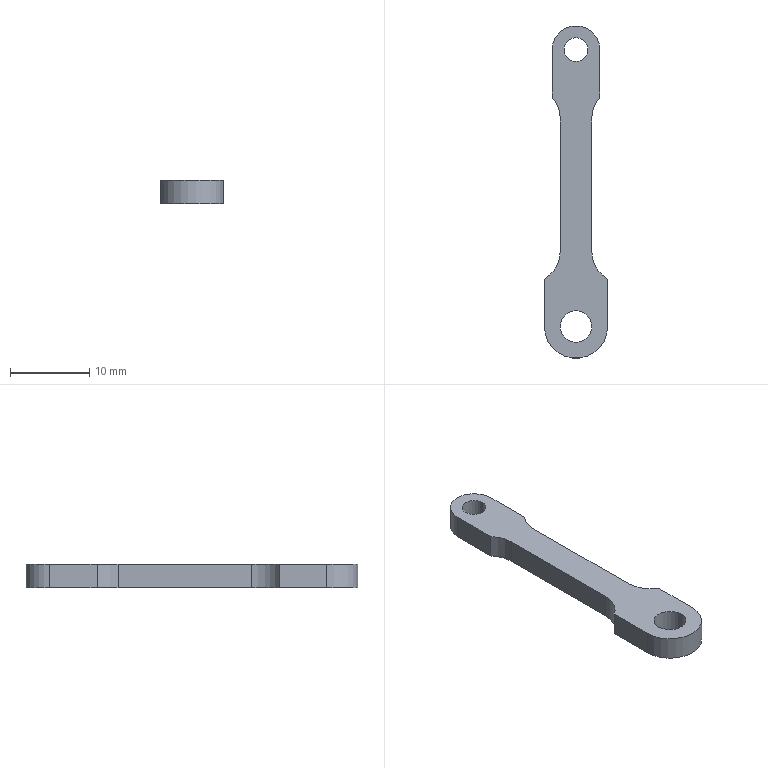Part | SolidWorks | features Extrusion 1 | 1 solid | 18 faces | box 8 x 42 x 3 mm | volume 603.988 mm3 | cylinder 10 | plane 8 | commonest cylinder face diameters 8 x5 3 x2 4 x2 6 x1
STEP:
#1=CARTESIAN_POINT('',(-2.,-35.,1.5));
#2=VERTEX_POINT('',#1);
#3=CARTESIAN_POINT('',(2.,-35.,1.5));
#4=VERTEX_POINT('',#3);
#5=CARTESIAN_POINT('',(0.,-35.,1.5));
#6=DIRECTION('',(0.,0.,1.));
#7=DIRECTION('',(1.,0.,0.));
#8=AXIS2_PLACEMENT_3D('',#5,#6,#7);
#9=CIRCLE('',#8,2.);
#10=EDGE_CURVE('',#2,#4,#9,.T.);
#11=ORIENTED_EDGE('',*,*,#10,.T.);
#12=CARTESIAN_POINT('',(2.,-35.,-1.5));
#13=VERTEX_POINT('',#12);
#14=CARTESIAN_POINT('',(2.,-35.,1.5));
#15=DIRECTION('',(0.,0.,-1.));
#16=VECTOR('',#15,1000.);
#17=LINE('',#14,#16);
#18=EDGE_CURVE('',#4,#13,#17,.T.);
#19=ORIENTED_EDGE('',*,*,#18,.T.);
#20=CARTESIAN_POINT('',(-2.,-35.,-1.5));
#21=VERTEX_POINT('',#20);
#22=CARTESIAN_POINT('',(0.,-35.,-1.5));
#23=DIRECTION('',(0.,0.,1.));
#24=DIRECTION('',(1.,0.,0.));
#25=AXIS2_PLACEMENT_3D('',#22,#23,#24);
#26=CIRCLE('',#25,2.);
#27=EDGE_CURVE('',#21,#13,#26,.T.);
#28=ORIENTED_EDGE('',*,*,#27,.F.);
#29=CARTESIAN_POINT('',(-2.,-35.,1.5));
#30=DIRECTION('',(0.,0.,-1.));
#31=VECTOR('',#30,1000.);
#32=LINE('',#29,#31);
#33=EDGE_CURVE('',#2,#21,#32,.T.);
#34=ORIENTED_EDGE('',*,*,#33,.F.);
#35=EDGE_LOOP('',(#11,#19,#28,#34));
#36=FACE_OUTER_BOUND('',#35,.T.);
#37=CARTESIAN_POINT('',(0.,-35.,1.5));
#38=DIRECTION('',(0.,0.,-1.));
#39=DIRECTION('',(-1.,0.,0.));
#40=AXIS2_PLACEMENT_3D('',#37,#38,#39);
#41=CYLINDRICAL_SURFACE('',#40,2.);
#42=ADVANCED_FACE('',(#36),#41,.F.);
#43=CARTESIAN_POINT('',(-1.5,0.,1.5));
#44=VERTEX_POINT('',#43);
#45=CARTESIAN_POINT('',(1.5,0.,1.5));
#46=VERTEX_POINT('',#45);
#47=CARTESIAN_POINT('',(0.,0.,1.5));
#48=DIRECTION('',(0.,0.,1.));
#49=DIRECTION('',(1.,0.,0.));
#50=AXIS2_PLACEMENT_3D('',#47,#48,#49);
#51=CIRCLE('',#50,1.5);
#52=EDGE_CURVE('',#44,#46,#51,.T.);
#53=ORIENTED_EDGE('',*,*,#52,.T.);
#54=CARTESIAN_POINT('',(1.5,0.,-1.5));
#55=VERTEX_POINT('',#54);
#56=CARTESIAN_POINT('',(1.5,0.,1.5));
#57=DIRECTION('',(0.,0.,-1.));
#58=VECTOR('',#57,1000.);
#59=LINE('',#56,#58);
#60=EDGE_CURVE('',#46,#55,#59,.T.);
#61=ORIENTED_EDGE('',*,*,#60,.T.);
#62=CARTESIAN_POINT('',(-1.5,0.,-1.5));
#63=VERTEX_POINT('',#62);
#64=CARTESIAN_POINT('',(0.,0.,-1.5));
#65=DIRECTION('',(0.,0.,1.));
#66=DIRECTION('',(1.,0.,0.));
#67=AXIS2_PLACEMENT_3D('',#64,#65,#66);
#68=CIRCLE('',#67,1.5);
#69=EDGE_CURVE('',#63,#55,#68,.T.);
#70=ORIENTED_EDGE('',*,*,#69,.F.);
#71=CARTESIAN_POINT('',(-1.5,0.,1.5));
#72=DIRECTION('',(0.,0.,-1.));
#73=VECTOR('',#72,1000.);
#74=LINE('',#71,#73);
#75=EDGE_CURVE('',#44,#63,#74,.T.);
#76=ORIENTED_EDGE('',*,*,#75,.F.);
#77=EDGE_LOOP('',(#53,#61,#70,#76));
#78=FACE_OUTER_BOUND('',#77,.T.);
#79=CARTESIAN_POINT('',(0.,0.,1.5));
#80=DIRECTION('',(0.,0.,-1.));
#81=DIRECTION('',(-1.,0.,0.));
#82=AXIS2_PLACEMENT_3D('',#79,#80,#81);
#83=CYLINDRICAL_SURFACE('',#82,1.5);
#84=ADVANCED_FACE('',(#78),#83,.F.);
#85=ORIENTED_EDGE('',*,*,#52,.F.);
#86=CARTESIAN_POINT('',(0.,0.,1.5));
#87=DIRECTION('',(0.,0.,1.));
#88=DIRECTION('',(1.,0.,0.));
#89=AXIS2_PLACEMENT_3D('',#86,#87,#88);
#90=CIRCLE('',#89,1.5);
#91=EDGE_CURVE('',#46,#44,#90,.T.);
#92=ORIENTED_EDGE('',*,*,#91,.F.);
#93=EDGE_LOOP('',(#85,#92));
#94=FACE_BOUND('',#93,.T.);
#95=CARTESIAN_POINT('',(3.,0.,1.5));
#96=VERTEX_POINT('',#95);
#97=CARTESIAN_POINT('',(-3.,0.,1.5));
#98=VERTEX_POINT('',#97);
#99=CARTESIAN_POINT('',(0.,0.,1.5));
#100=DIRECTION('',(0.,0.,1.));
#101=DIRECTION('',(1.,0.,0.));
#102=AXIS2_PLACEMENT_3D('',#99,#100,#101);
#103=CIRCLE('',#102,3.);
#104=EDGE_CURVE('',#96,#98,#103,.T.);
#105=ORIENTED_EDGE('',*,*,#104,.T.);
#106=CARTESIAN_POINT('',(-3.,-6.,1.5));
#107=VERTEX_POINT('',#106);
#108=CARTESIAN_POINT('',(-3.,0.,1.5));
#109=DIRECTION('',(0.,-1.,0.));
#110=VECTOR('',#109,1000.);
#111=LINE('',#108,#110);
#112=EDGE_CURVE('',#98,#107,#111,.T.);
#113=ORIENTED_EDGE('',*,*,#112,.T.);
#114=CARTESIAN_POINT('',(-2.,-8.646,1.5));
#115=VERTEX_POINT('',#114);
#116=CARTESIAN_POINT('',(-6.,-8.646,1.5));
#117=DIRECTION('',(0.,0.,-1.));
#118=DIRECTION('',(1.,0.,0.));
#119=AXIS2_PLACEMENT_3D('',#116,#117,#118);
#120=CIRCLE('',#119,4.);
#121=EDGE_CURVE('',#107,#115,#120,.T.);
#122=ORIENTED_EDGE('',*,*,#121,.T.);
#123=CARTESIAN_POINT('',(-2.,-25.536,1.5));
#124=VERTEX_POINT('',#123);
#125=CARTESIAN_POINT('',(-2.,-8.646,1.5));
#126=DIRECTION('',(0.,-1.,0.));
#127=VECTOR('',#126,1000.);
#128=LINE('',#125,#127);
#129=EDGE_CURVE('',#115,#124,#128,.T.);
#130=ORIENTED_EDGE('',*,*,#129,.T.);
#131=CARTESIAN_POINT('',(-4.,-29.,1.5));
#132=VERTEX_POINT('',#131);
#133=CARTESIAN_POINT('',(-6.,-25.536,1.5));
#134=DIRECTION('',(0.,0.,-1.));
#135=DIRECTION('',(1.,0.,0.));
#136=AXIS2_PLACEMENT_3D('',#133,#134,#135);
#137=CIRCLE('',#136,4.);
#138=EDGE_CURVE('',#124,#132,#137,.T.);
#139=ORIENTED_EDGE('',*,*,#138,.T.);
#140=CARTESIAN_POINT('',(-4.,-35.,1.5));
#141=VERTEX_POINT('',#140);
#142=CARTESIAN_POINT('',(-4.,-35.,1.5));
#143=DIRECTION('',(0.,-1.,0.));
#144=VECTOR('',#143,1000.);
#145=LINE('',#142,#144);
#146=EDGE_CURVE('',#132,#141,#145,.T.);
#147=ORIENTED_EDGE('',*,*,#146,.T.);
#148=CARTESIAN_POINT('',(4.,-35.,1.5));
#149=VERTEX_POINT('',#148);
#150=CARTESIAN_POINT('',(0.,-35.,1.5));
#151=DIRECTION('',(0.,0.,1.));
#152=DIRECTION('',(1.,0.,0.));
#153=AXIS2_PLACEMENT_3D('',#150,#151,#152);
#154=CIRCLE('',#153,4.);
#155=EDGE_CURVE('',#141,#149,#154,.T.);
#156=ORIENTED_EDGE('',*,*,#155,.T.);
#157=CARTESIAN_POINT('',(4.,-29.,1.5));
#158=VERTEX_POINT('',#157);
#159=CARTESIAN_POINT('',(4.,-35.,1.5));
#160=DIRECTION('',(0.,1.,0.));
#161=VECTOR('',#160,1000.);
#162=LINE('',#159,#161);
#163=EDGE_CURVE('',#149,#158,#162,.T.);
#164=ORIENTED_EDGE('',*,*,#163,.T.);
#165=CARTESIAN_POINT('',(2.,-25.536,1.5));
#166=VERTEX_POINT('',#165);
#167=CARTESIAN_POINT('',(6.,-25.536,1.5));
#168=DIRECTION('',(0.,0.,-1.));
#169=DIRECTION('',(-1.,0.,0.));
#170=AXIS2_PLACEMENT_3D('',#167,#168,#169);
#171=CIRCLE('',#170,4.);
#172=EDGE_CURVE('',#158,#166,#171,.T.);
#173=ORIENTED_EDGE('',*,*,#172,.T.);
#174=CARTESIAN_POINT('',(2.,-8.646,1.5));
#175=VERTEX_POINT('',#174);
#176=CARTESIAN_POINT('',(2.,-8.646,1.5));
#177=DIRECTION('',(0.,1.,0.));
#178=VECTOR('',#177,1000.);
#179=LINE('',#176,#178);
#180=EDGE_CURVE('',#166,#175,#179,.T.);
#181=ORIENTED_EDGE('',*,*,#180,.T.);
#182=CARTESIAN_POINT('',(3.,-6.,1.5));
#183=VERTEX_POINT('',#182);
#184=CARTESIAN_POINT('',(6.,-8.646,1.5));
#185=DIRECTION('',(0.,0.,-1.));
#186=DIRECTION('',(-1.,0.,0.));
#187=AXIS2_PLACEMENT_3D('',#184,#185,#186);
#188=CIRCLE('',#187,4.);
#189=EDGE_CURVE('',#175,#183,#188,.T.);
#190=ORIENTED_EDGE('',*,*,#189,.T.);
#191=CARTESIAN_POINT('',(3.,0.,1.5));
#192=DIRECTION('',(0.,1.,0.));
#193=VECTOR('',#192,1000.);
#194=LINE('',#191,#193);
#195=EDGE_CURVE('',#183,#96,#194,.T.);
#196=ORIENTED_EDGE('',*,*,#195,.T.);
#197=EDGE_LOOP('',(#105,#113,#122,#130,#139,#147,#156,#164,#173,#181,#190,#196));
#198=FACE_OUTER_BOUND('',#197,.T.);
#199=ORIENTED_EDGE('',*,*,#10,.F.);
#200=CARTESIAN_POINT('',(0.,-35.,1.5));
#201=DIRECTION('',(0.,0.,1.));
#202=DIRECTION('',(1.,0.,0.));
#203=AXIS2_PLACEMENT_3D('',#200,#201,#202);
#204=CIRCLE('',#203,2.);
#205=EDGE_CURVE('',#4,#2,#204,.T.);
#206=ORIENTED_EDGE('',*,*,#205,.F.);
#207=EDGE_LOOP('',(#199,#206));
#208=FACE_BOUND('',#207,.T.);
#209=CARTESIAN_POINT('',(0.,0.,1.5));
#210=DIRECTION('',(0.,0.,1.));
#211=DIRECTION('',(1.,0.,0.));
#212=AXIS2_PLACEMENT_3D('',#209,#210,#211);
#213=PLANE('',#212);
#214=ADVANCED_FACE('',(#94,#198,#208),#213,.T.);
#215=CARTESIAN_POINT('',(3.,0.,-1.5));
#216=VERTEX_POINT('',#215);
#217=CARTESIAN_POINT('',(-3.,0.,-1.5));
#218=VERTEX_POINT('',#217);
#219=CARTESIAN_POINT('',(0.,0.,-1.5));
#220=DIRECTION('',(0.,0.,1.));
#221=DIRECTION('',(1.,0.,0.));
#222=AXIS2_PLACEMENT_3D('',#219,#220,#221);
#223=CIRCLE('',#222,3.);
#224=EDGE_CURVE('',#216,#218,#223,.T.);
#225=ORIENTED_EDGE('',*,*,#224,.F.);
#226=CARTESIAN_POINT('',(3.,-6.,-1.5));
#227=VERTEX_POINT('',#226);
#228=CARTESIAN_POINT('',(3.,0.,-1.5));
#229=DIRECTION('',(0.,1.,0.));
#230=VECTOR('',#229,1000.);
#231=LINE('',#228,#230);
#232=EDGE_CURVE('',#227,#216,#231,.T.);
#233=ORIENTED_EDGE('',*,*,#232,.F.);
#234=CARTESIAN_POINT('',(2.,-8.646,-1.5));
#235=VERTEX_POINT('',#234);
#236=CARTESIAN_POINT('',(6.,-8.646,-1.5));
#237=DIRECTION('',(0.,0.,-1.));
#238=DIRECTION('',(-1.,0.,0.));
#239=AXIS2_PLACEMENT_3D('',#236,#237,#238);
#240=CIRCLE('',#239,4.);
#241=EDGE_CURVE('',#235,#227,#240,.T.);
#242=ORIENTED_EDGE('',*,*,#241,.F.);
#243=CARTESIAN_POINT('',(2.,-25.536,-1.5));
#244=VERTEX_POINT('',#243);
#245=CARTESIAN_POINT('',(2.,-8.646,-1.5));
#246=DIRECTION('',(0.,1.,0.));
#247=VECTOR('',#246,1000.);
#248=LINE('',#245,#247);
#249=EDGE_CURVE('',#244,#235,#248,.T.);
#250=ORIENTED_EDGE('',*,*,#249,.F.);
#251=CARTESIAN_POINT('',(4.,-29.,-1.5));
#252=VERTEX_POINT('',#251);
#253=CARTESIAN_POINT('',(6.,-25.536,-1.5));
#254=DIRECTION('',(0.,0.,-1.));
#255=DIRECTION('',(-1.,0.,0.));
#256=AXIS2_PLACEMENT_3D('',#253,#254,#255);
#257=CIRCLE('',#256,4.);
#258=EDGE_CURVE('',#252,#244,#257,.T.);
#259=ORIENTED_EDGE('',*,*,#258,.F.);
#260=CARTESIAN_POINT('',(4.,-35.,-1.5));
#261=VERTEX_POINT('',#260);
#262=CARTESIAN_POINT('',(4.,-35.,-1.5));
#263=DIRECTION('',(0.,1.,0.));
#264=VECTOR('',#263,1000.);
#265=LINE('',#262,#264);
#266=EDGE_CURVE('',#261,#252,#265,.T.);
#267=ORIENTED_EDGE('',*,*,#266,.F.);
#268=CARTESIAN_POINT('',(-4.,-35.,-1.5));
#269=VERTEX_POINT('',#268);
#270=CARTESIAN_POINT('',(0.,-35.,-1.5));
#271=DIRECTION('',(0.,0.,1.));
#272=DIRECTION('',(1.,0.,0.));
#273=AXIS2_PLACEMENT_3D('',#270,#271,#272);
#274=CIRCLE('',#273,4.);
#275=EDGE_CURVE('',#269,#261,#274,.T.);
#276=ORIENTED_EDGE('',*,*,#275,.F.);
#277=CARTESIAN_POINT('',(-4.,-29.,-1.5));
#278=VERTEX_POINT('',#277);
#279=CARTESIAN_POINT('',(-4.,-35.,-1.5));
#280=DIRECTION('',(0.,-1.,0.));
#281=VECTOR('',#280,1000.);
#282=LINE('',#279,#281);
#283=EDGE_CURVE('',#278,#269,#282,.T.);
#284=ORIENTED_EDGE('',*,*,#283,.F.);
#285=CARTESIAN_POINT('',(-2.,-25.536,-1.5));
#286=VERTEX_POINT('',#285);
#287=CARTESIAN_POINT('',(-6.,-25.536,-1.5));
#288=DIRECTION('',(0.,0.,-1.));
#289=DIRECTION('',(1.,0.,0.));
#290=AXIS2_PLACEMENT_3D('',#287,#288,#289);
#291=CIRCLE('',#290,4.);
#292=EDGE_CURVE('',#286,#278,#291,.T.);
#293=ORIENTED_EDGE('',*,*,#292,.F.);
#294=CARTESIAN_POINT('',(-2.,-8.646,-1.5));
#295=VERTEX_POINT('',#294);
#296=CARTESIAN_POINT('',(-2.,-8.646,-1.5));
#297=DIRECTION('',(0.,-1.,0.));
#298=VECTOR('',#297,1000.);
#299=LINE('',#296,#298);
#300=EDGE_CURVE('',#295,#286,#299,.T.);
#301=ORIENTED_EDGE('',*,*,#300,.F.);
#302=CARTESIAN_POINT('',(-3.,-6.,-1.5));
#303=VERTEX_POINT('',#302);
#304=CARTESIAN_POINT('',(-6.,-8.646,-1.5));
#305=DIRECTION('',(0.,0.,-1.));
#306=DIRECTION('',(1.,0.,0.));
#307=AXIS2_PLACEMENT_3D('',#304,#305,#306);
#308=CIRCLE('',#307,4.);
#309=EDGE_CURVE('',#303,#295,#308,.T.);
#310=ORIENTED_EDGE('',*,*,#309,.F.);
#311=CARTESIAN_POINT('',(-3.,0.,-1.5));
#312=DIRECTION('',(0.,-1.,0.));
#313=VECTOR('',#312,1000.);
#314=LINE('',#311,#313);
#315=EDGE_CURVE('',#218,#303,#314,.T.);
#316=ORIENTED_EDGE('',*,*,#315,.F.);
#317=EDGE_LOOP('',(#225,#233,#242,#250,#259,#267,#276,#284,#293,#301,#310,#316));
#318=FACE_OUTER_BOUND('',#317,.T.);
#319=ORIENTED_EDGE('',*,*,#69,.T.);
#320=CARTESIAN_POINT('',(0.,0.,-1.5));
#321=DIRECTION('',(0.,0.,1.));
#322=DIRECTION('',(1.,0.,0.));
#323=AXIS2_PLACEMENT_3D('',#320,#321,#322);
#324=CIRCLE('',#323,1.5);
#325=EDGE_CURVE('',#55,#63,#324,.T.);
#326=ORIENTED_EDGE('',*,*,#325,.T.);
#327=EDGE_LOOP('',(#319,#326));
#328=FACE_BOUND('',#327,.T.);
#329=ORIENTED_EDGE('',*,*,#27,.T.);
#330=CARTESIAN_POINT('',(0.,-35.,-1.5));
#331=DIRECTION('',(0.,0.,1.));
#332=DIRECTION('',(1.,0.,0.));
#333=AXIS2_PLACEMENT_3D('',#330,#331,#332);
#334=CIRCLE('',#333,2.);
#335=EDGE_CURVE('',#13,#21,#334,.T.);
#336=ORIENTED_EDGE('',*,*,#335,.T.);
#337=EDGE_LOOP('',(#329,#336));
#338=FACE_BOUND('',#337,.T.);
#339=CARTESIAN_POINT('',(0.,0.,-1.5));
#340=DIRECTION('',(0.,0.,1.));
#341=DIRECTION('',(1.,0.,0.));
#342=AXIS2_PLACEMENT_3D('',#339,#340,#341);
#343=PLANE('',#342);
#344=ADVANCED_FACE('',(#318,#328,#338),#343,.F.);
#345=ORIENTED_EDGE('',*,*,#224,.T.);
#346=CARTESIAN_POINT('',(-3.,0.,1.5));
#347=DIRECTION('',(0.,0.,-1.));
#348=VECTOR('',#347,1000.);
#349=LINE('',#346,#348);
#350=EDGE_CURVE('',#98,#218,#349,.T.);
#351=ORIENTED_EDGE('',*,*,#350,.F.);
#352=ORIENTED_EDGE('',*,*,#104,.F.);
#353=CARTESIAN_POINT('',(3.,0.,1.5));
#354=DIRECTION('',(0.,0.,-1.));
#355=VECTOR('',#354,1000.);
#356=LINE('',#353,#355);
#357=EDGE_CURVE('',#96,#216,#356,.T.);
#358=ORIENTED_EDGE('',*,*,#357,.T.);
#359=EDGE_LOOP('',(#345,#351,#352,#358));
#360=FACE_OUTER_BOUND('',#359,.T.);
#361=CARTESIAN_POINT('',(0.,0.,1.5));
#362=DIRECTION('',(0.,0.,-1.));
#363=DIRECTION('',(-1.,0.,0.));
#364=AXIS2_PLACEMENT_3D('',#361,#362,#363);
#365=CYLINDRICAL_SURFACE('',#364,3.);
#366=ADVANCED_FACE('',(#360),#365,.T.);
#367=ORIENTED_EDGE('',*,*,#315,.T.);
#368=CARTESIAN_POINT('',(-3.,-6.,1.5));
#369=DIRECTION('',(0.,0.,-1.));
#370=VECTOR('',#369,1000.);
#371=LINE('',#368,#370);
#372=EDGE_CURVE('',#107,#303,#371,.T.);
#373=ORIENTED_EDGE('',*,*,#372,.F.);
#374=ORIENTED_EDGE('',*,*,#112,.F.);
#375=ORIENTED_EDGE('',*,*,#350,.T.);
#376=EDGE_LOOP('',(#367,#373,#374,#375));
#377=FACE_OUTER_BOUND('',#376,.T.);
#378=CARTESIAN_POINT('',(-3.,0.,1.5));
#379=DIRECTION('',(1.,0.,0.));
#380=DIRECTION('',(0.,1.,0.));
#381=AXIS2_PLACEMENT_3D('',#378,#379,#380);
#382=PLANE('',#381);
#383=ADVANCED_FACE('',(#377),#382,.F.);
#384=ORIENTED_EDGE('',*,*,#309,.T.);
#385=CARTESIAN_POINT('',(-2.,-8.646,1.5));
#386=DIRECTION('',(0.,0.,-1.));
#387=VECTOR('',#386,1000.);
#388=LINE('',#385,#387);
#389=EDGE_CURVE('',#115,#295,#388,.T.);
#390=ORIENTED_EDGE('',*,*,#389,.F.);
#391=ORIENTED_EDGE('',*,*,#121,.F.);
#392=ORIENTED_EDGE('',*,*,#372,.T.);
#393=EDGE_LOOP('',(#384,#390,#391,#392));
#394=FACE_OUTER_BOUND('',#393,.T.);
#395=CARTESIAN_POINT('',(-6.,-8.646,1.5));
#396=DIRECTION('',(0.,0.,-1.));
#397=DIRECTION('',(-1.,0.,0.));
#398=AXIS2_PLACEMENT_3D('',#395,#396,#397);
#399=CYLINDRICAL_SURFACE('',#398,4.);
#400=ADVANCED_FACE('',(#394),#399,.F.);
#401=ORIENTED_EDGE('',*,*,#300,.T.);
#402=CARTESIAN_POINT('',(-2.,-25.536,1.5));
#403=DIRECTION('',(0.,0.,-1.));
#404=VECTOR('',#403,1000.);
#405=LINE('',#402,#404);
#406=EDGE_CURVE('',#124,#286,#405,.T.);
#407=ORIENTED_EDGE('',*,*,#406,.F.);
#408=ORIENTED_EDGE('',*,*,#129,.F.);
#409=ORIENTED_EDGE('',*,*,#389,.T.);
#410=EDGE_LOOP('',(#401,#407,#408,#409));
#411=FACE_OUTER_BOUND('',#410,.T.);
#412=CARTESIAN_POINT('',(-2.,-8.646,1.5));
#413=DIRECTION('',(1.,0.,0.));
#414=DIRECTION('',(0.,1.,0.));
#415=AXIS2_PLACEMENT_3D('',#412,#413,#414);
#416=PLANE('',#415);
#417=ADVANCED_FACE('',(#411),#416,.F.);
#418=ORIENTED_EDGE('',*,*,#292,.T.);
#419=CARTESIAN_POINT('',(-4.,-29.,1.5));
#420=DIRECTION('',(0.,0.,-1.));
#421=VECTOR('',#420,1000.);
#422=LINE('',#419,#421);
#423=EDGE_CURVE('',#132,#278,#422,.T.);
#424=ORIENTED_EDGE('',*,*,#423,.F.);
#425=ORIENTED_EDGE('',*,*,#138,.F.);
#426=ORIENTED_EDGE('',*,*,#406,.T.);
#427=EDGE_LOOP('',(#418,#424,#425,#426));
#428=FACE_OUTER_BOUND('',#427,.T.);
#429=CARTESIAN_POINT('',(-6.,-25.536,1.5));
#430=DIRECTION('',(0.,0.,-1.));
#431=DIRECTION('',(-1.,0.,0.));
#432=AXIS2_PLACEMENT_3D('',#429,#430,#431);
#433=CYLINDRICAL_SURFACE('',#432,4.);
#434=ADVANCED_FACE('',(#428),#433,.F.);
#435=ORIENTED_EDGE('',*,*,#283,.T.);
#436=CARTESIAN_POINT('',(-4.,-35.,1.5));
#437=DIRECTION('',(0.,0.,-1.));
#438=VECTOR('',#437,1000.);
#439=LINE('',#436,#438);
#440=EDGE_CURVE('',#141,#269,#439,.T.);
#441=ORIENTED_EDGE('',*,*,#440,.F.);
#442=ORIENTED_EDGE('',*,*,#146,.F.);
#443=ORIENTED_EDGE('',*,*,#423,.T.);
#444=EDGE_LOOP('',(#435,#441,#442,#443));
#445=FACE_OUTER_BOUND('',#444,.T.);
#446=CARTESIAN_POINT('',(-4.,-35.,1.5));
#447=DIRECTION('',(1.,0.,0.));
#448=DIRECTION('',(0.,0.,-1.));
#449=AXIS2_PLACEMENT_3D('',#446,#447,#448);
#450=PLANE('',#449);
#451=ADVANCED_FACE('',(#445),#450,.F.);
#452=ORIENTED_EDGE('',*,*,#275,.T.);
#453=CARTESIAN_POINT('',(4.,-35.,1.5));
#454=DIRECTION('',(0.,0.,-1.));
#455=VECTOR('',#454,1000.);
#456=LINE('',#453,#455);
#457=EDGE_CURVE('',#149,#261,#456,.T.);
#458=ORIENTED_EDGE('',*,*,#457,.F.);
#459=ORIENTED_EDGE('',*,*,#155,.F.);
#460=ORIENTED_EDGE('',*,*,#440,.T.);
#461=EDGE_LOOP('',(#452,#458,#459,#460));
#462=FACE_OUTER_BOUND('',#461,.T.);
#463=CARTESIAN_POINT('',(0.,-35.,1.5));
#464=DIRECTION('',(0.,0.,-1.));
#465=DIRECTION('',(-1.,0.,0.));
#466=AXIS2_PLACEMENT_3D('',#463,#464,#465);
#467=CYLINDRICAL_SURFACE('',#466,4.);
#468=ADVANCED_FACE('',(#462),#467,.T.);
#469=ORIENTED_EDGE('',*,*,#266,.T.);
#470=CARTESIAN_POINT('',(4.,-29.,1.5));
#471=DIRECTION('',(0.,0.,-1.));
#472=VECTOR('',#471,1000.);
#473=LINE('',#470,#472);
#474=EDGE_CURVE('',#158,#252,#473,.T.);
#475=ORIENTED_EDGE('',*,*,#474,.F.);
#476=ORIENTED_EDGE('',*,*,#163,.F.);
#477=ORIENTED_EDGE('',*,*,#457,.T.);
#478=EDGE_LOOP('',(#469,#475,#476,#477));
#479=FACE_OUTER_BOUND('',#478,.T.);
#480=CARTESIAN_POINT('',(4.,-35.,1.5));
#481=DIRECTION('',(-1.,0.,0.));
#482=DIRECTION('',(0.,-1.,0.));
#483=AXIS2_PLACEMENT_3D('',#480,#481,#482);
#484=PLANE('',#483);
#485=ADVANCED_FACE('',(#479),#484,.F.);
#486=ORIENTED_EDGE('',*,*,#258,.T.);
#487=CARTESIAN_POINT('',(2.,-25.536,1.5));
#488=DIRECTION('',(0.,0.,-1.));
#489=VECTOR('',#488,1000.);
#490=LINE('',#487,#489);
#491=EDGE_CURVE('',#166,#244,#490,.T.);
#492=ORIENTED_EDGE('',*,*,#491,.F.);
#493=ORIENTED_EDGE('',*,*,#172,.F.);
#494=ORIENTED_EDGE('',*,*,#474,.T.);
#495=EDGE_LOOP('',(#486,#492,#493,#494));
#496=FACE_OUTER_BOUND('',#495,.T.);
#497=CARTESIAN_POINT('',(6.,-25.536,1.5));
#498=DIRECTION('',(0.,0.,-1.));
#499=DIRECTION('',(-1.,0.,0.));
#500=AXIS2_PLACEMENT_3D('',#497,#498,#499);
#501=CYLINDRICAL_SURFACE('',#500,4.);
#502=ADVANCED_FACE('',(#496),#501,.F.);
#503=ORIENTED_EDGE('',*,*,#249,.T.);
#504=CARTESIAN_POINT('',(2.,-8.646,1.5));
#505=DIRECTION('',(0.,0.,-1.));
#506=VECTOR('',#505,1000.);
#507=LINE('',#504,#506);
#508=EDGE_CURVE('',#175,#235,#507,.T.);
#509=ORIENTED_EDGE('',*,*,#508,.F.);
#510=ORIENTED_EDGE('',*,*,#180,.F.);
#511=ORIENTED_EDGE('',*,*,#491,.T.);
#512=EDGE_LOOP('',(#503,#509,#510,#511));
#513=FACE_OUTER_BOUND('',#512,.T.);
#514=CARTESIAN_POINT('',(2.,-8.646,1.5));
#515=DIRECTION('',(-1.,0.,0.));
#516=DIRECTION('',(0.,-1.,0.));
#517=AXIS2_PLACEMENT_3D('',#514,#515,#516);
#518=PLANE('',#517);
#519=ADVANCED_FACE('',(#513),#518,.F.);
#520=ORIENTED_EDGE('',*,*,#241,.T.);
#521=CARTESIAN_POINT('',(3.,-6.,1.5));
#522=DIRECTION('',(0.,0.,-1.));
#523=VECTOR('',#522,1000.);
#524=LINE('',#521,#523);
#525=EDGE_CURVE('',#183,#227,#524,.T.);
#526=ORIENTED_EDGE('',*,*,#525,.F.);
#527=ORIENTED_EDGE('',*,*,#189,.F.);
#528=ORIENTED_EDGE('',*,*,#508,.T.);
#529=EDGE_LOOP('',(#520,#526,#527,#528));
#530=FACE_OUTER_BOUND('',#529,.T.);
#531=CARTESIAN_POINT('',(6.,-8.646,1.5));
#532=DIRECTION('',(0.,0.,-1.));
#533=DIRECTION('',(-1.,0.,0.));
#534=AXIS2_PLACEMENT_3D('',#531,#532,#533);
#535=CYLINDRICAL_SURFACE('',#534,4.);
#536=ADVANCED_FACE('',(#530),#535,.F.);
#537=ORIENTED_EDGE('',*,*,#232,.T.);
#538=ORIENTED_EDGE('',*,*,#357,.F.);
#539=ORIENTED_EDGE('',*,*,#195,.F.);
#540=ORIENTED_EDGE('',*,*,#525,.T.);
#541=EDGE_LOOP('',(#537,#538,#539,#540));
#542=FACE_OUTER_BOUND('',#541,.T.);
#543=CARTESIAN_POINT('',(3.,0.,1.5));
#544=DIRECTION('',(-1.,0.,0.));
#545=DIRECTION('',(0.,-1.,0.));
#546=AXIS2_PLACEMENT_3D('',#543,#544,#545);
#547=PLANE('',#546);
#548=ADVANCED_FACE('',(#542),#547,.F.);
#549=ORIENTED_EDGE('',*,*,#60,.F.);
#550=ORIENTED_EDGE('',*,*,#91,.T.);
#551=ORIENTED_EDGE('',*,*,#75,.T.);
#552=ORIENTED_EDGE('',*,*,#325,.F.);
#553=EDGE_LOOP('',(#549,#550,#551,#552));
#554=FACE_OUTER_BOUND('',#553,.T.);
#555=CARTESIAN_POINT('',(0.,0.,1.5));
#556=DIRECTION('',(0.,0.,-1.));
#557=DIRECTION('',(-1.,0.,0.));
#558=AXIS2_PLACEMENT_3D('',#555,#556,#557);
#559=CYLINDRICAL_SURFACE('',#558,1.5);
#560=ADVANCED_FACE('',(#554),#559,.F.);
#561=ORIENTED_EDGE('',*,*,#18,.F.);
#562=ORIENTED_EDGE('',*,*,#205,.T.);
#563=ORIENTED_EDGE('',*,*,#33,.T.);
#564=ORIENTED_EDGE('',*,*,#335,.F.);
#565=EDGE_LOOP('',(#561,#562,#563,#564));
#566=FACE_OUTER_BOUND('',#565,.T.);
#567=CARTESIAN_POINT('',(0.,-35.,1.5));
#568=DIRECTION('',(0.,0.,-1.));
#569=DIRECTION('',(-1.,0.,0.));
#570=AXIS2_PLACEMENT_3D('',#567,#568,#569);
#571=CYLINDRICAL_SURFACE('',#570,2.);
#572=ADVANCED_FACE('',(#566),#571,.F.);
#573=CLOSED_SHELL('',(#42,#84,#214,#344,#366,#383,#400,#417,#434,#451,#468,#485,#502,#519,#536,#548,#560,#572));
#574=MANIFOLD_SOLID_BREP('',#573);
#575=CARTESIAN_POINT('',(0.,0.,0.));
#576=DIRECTION('',(0.,0.,1.));
#577=DIRECTION('',(1.,0.,0.));
#578=AXIS2_PLACEMENT_3D('',#575,#576,#577);
#579=(LENGTH_UNIT()NAMED_UNIT(*)SI_UNIT(.MILLI.,.METRE.));
#580=UNCERTAINTY_MEASURE_WITH_UNIT(LENGTH_MEASURE(0.00001),#579,'','');
#581=(NAMED_UNIT(*)PLANE_ANGLE_UNIT()SI_UNIT($,.RADIAN.));
#582=(NAMED_UNIT(*)SI_UNIT($,.STERADIAN.)SOLID_ANGLE_UNIT());
#583=(GEOMETRIC_REPRESENTATION_CONTEXT(3)GLOBAL_UNCERTAINTY_ASSIGNED_CONTEXT((#580))GLOBAL_UNIT_ASSIGNED_CONTEXT((#579,#581,#582))REPRESENTATION_CONTEXT('',''));
#584=ADVANCED_BREP_SHAPE_REPRESENTATION('',(#574,#578),#583);